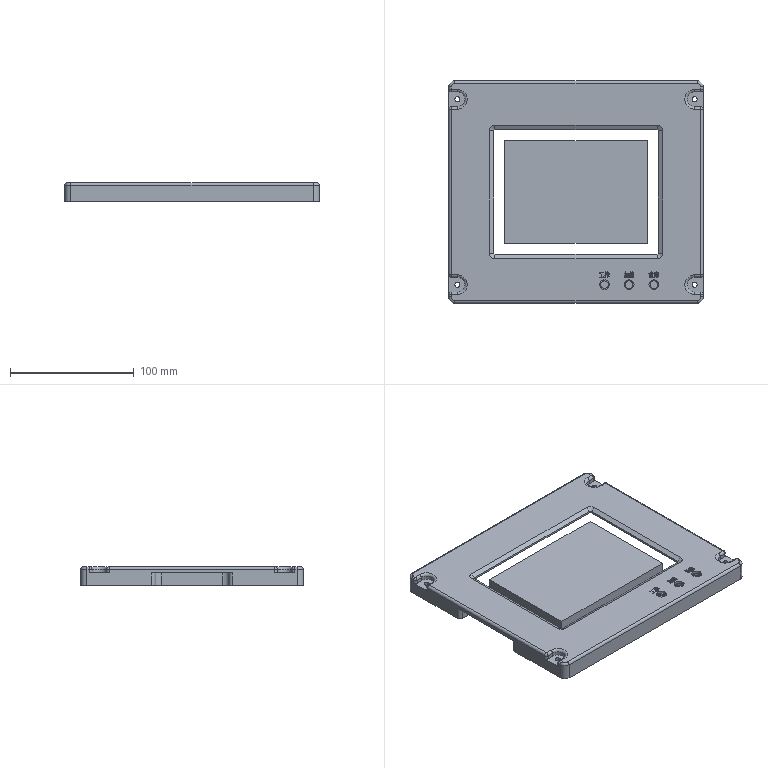NC program | Mastercam | posted with a generic post | part box 206 x 180 x 15 mm
Lines 14414 to 15524 of 42274:
(2 BM/BNOS |TOOL - 14|DIA. OFF. - 14|LEN. - 14|TOOL DIA. - 2.)
N9094 T14 M6
N9096 G0 G54 G90 X69.714 Y49.5 C0. B0. S10000 M3
N9098 G43 H14 Z24.866
N9100 Z4.866
N9102 G1 Z-.134 F600.
N9104 X69.698 Y49.856 F2000.
N9106 X69.648 Y50.221
N9108 X69.561 Y50.591
N9110 X69.436 Y50.959
N9112 X69.271 Y51.321
N9114 X69.068 Y51.669
N9116 X68.828 Y51.999
N9118 X68.553 Y52.303
N9120 X68.249 Y52.578
N9122 X67.919 Y52.818
N9124 X67.571 Y53.021
N9126 X67.209 Y53.186
N9128 X66.841 Y53.311
N9130 X66.471 Y53.398
N9132 X66.106 Y53.448
N9134 X65.75 Y53.464
N9136 X-65.75
N9138 X-66.106 Y53.448
N9140 X-66.471 Y53.398
N9142 X-66.841 Y53.311
N9144 X-67.209 Y53.186
N9146 X-67.571 Y53.021
N9148 X-67.919 Y52.818
N9150 X-68.249 Y52.578
N9152 X-68.553 Y52.303
N9154 X-68.828 Y51.999
N9156 X-69.068 Y51.669
N9158 X-69.271 Y51.321
N9160 X-69.436 Y50.959
N9162 X-69.561 Y50.591
N9164 X-69.648 Y50.221
N9166 X-69.698 Y49.856
N9168 X-69.714 Y49.5
N9170 Y-49.5
N9172 X-69.627
N9174 Z-.184
N9176 Y49.5
N9178 X-69.612 Y49.848
N9180 X-69.563 Y50.206
N9182 X-69.478 Y50.567
N9184 X-69.355 Y50.927
N9186 X-69.194 Y51.281
N9188 X-68.995 Y51.622
N9190 X-68.76 Y51.944
N9192 X-68.492 Y52.242
N9194 X-68.194 Y52.51
N9196 X-67.872 Y52.745
N9198 X-67.531 Y52.944
N9200 X-67.177 Y53.105
N9202 X-66.817 Y53.228
N9204 X-66.456 Y53.313
N9206 X-66.098 Y53.362
N9208 X-65.75 Y53.377
N9210 X65.75
N9212 X66.098 Y53.362
N9214 X66.456 Y53.313
N9216 X66.817 Y53.228
N9218 X67.177 Y53.105
N9220 X67.531 Y52.944
N9222 X67.872 Y52.745
N9224 X68.194 Y52.51
N9226 X68.492 Y52.242
N9228 X68.76 Y51.944
N9230 X68.995 Y51.622
N9232 X69.194 Y51.281
N9234 X69.355 Y50.927
N9236 X69.478 Y50.567
N9238 X69.563 Y50.206
N9240 X69.612 Y49.848
N9242 X69.627 Y49.5
N9244 Y-49.5
N9246 X69.612 Y-49.848
N9248 X69.563 Y-50.206
N9250 X69.478 Y-50.567
N9252 X69.355 Y-50.927
N9254 X69.194 Y-51.281
N9256 X68.995 Y-51.622
N9258 X68.76 Y-51.944
N9260 X68.492 Y-52.242
N9262 X68.194 Y-52.51
N9264 X67.872 Y-52.745
N9266 X67.531 Y-52.944
N9268 X67.177 Y-53.105
N9270 X66.817 Y-53.228
N9272 X66.456 Y-53.313
N9274 X66.098 Y-53.362
N9276 X65.75 Y-53.377
N9278 X-65.75
N9280 X-66.098 Y-53.362
N9282 X-66.456 Y-53.313
N9284 X-66.817 Y-53.228
N9286 X-67.177 Y-53.105
N9288 X-67.531 Y-52.944
N9290 X-67.872 Y-52.745
N9292 X-68.194 Y-52.51
N9294 X-68.492 Y-52.242
N9296 X-68.76 Y-51.944
N9298 X-68.995 Y-51.622
N9300 X-69.194 Y-51.281
N9302 X-69.355 Y-50.927
N9304 X-69.478 Y-50.567
N9306 X-69.563 Y-50.206
N9308 X-69.612 Y-49.848
N9310 X-69.627 Y-49.5
N9312 X-69.541
N9314 Z-.234
N9316 X-69.526 Y-49.841
N9318 X-69.478 Y-50.19
N9320 X-69.395 Y-50.543
N9322 X-69.275 Y-50.895
N9324 X-69.117 Y-51.241
N9326 X-68.923 Y-51.574
N9328 X-68.693 Y-51.889
N9330 X-68.431 Y-52.181
N9332 X-68.139 Y-52.443
N9334 X-67.824 Y-52.673
N9336 X-67.491 Y-52.867
N9338 X-67.145 Y-53.025
N9340 X-66.793 Y-53.145
N9342 X-66.44 Y-53.228
N9344 X-66.091 Y-53.276
N9346 X-65.75 Y-53.291
N9348 X65.75
N9350 X66.091 Y-53.276
N9352 X66.44 Y-53.228
N9354 X66.793 Y-53.145
N9356 X67.145 Y-53.025
N9358 X67.491 Y-52.867
N9360 X67.824 Y-52.673
N9362 X68.139 Y-52.443
N9364 X68.431 Y-52.181
N9366 X68.693 Y-51.889
N9368 X68.923 Y-51.574
N9370 X69.117 Y-51.241
N9372 X69.275 Y-50.895
N9374 X69.395 Y-50.543
N9376 X69.478 Y-50.19
N9378 X69.526 Y-49.841
N9380 X69.541 Y-49.5
N9382 Y49.5
N9384 X69.526 Y49.841
N9386 X69.478 Y50.19
N9388 X69.395 Y50.543
N9390 X69.275 Y50.895
N9392 X69.117 Y51.241
N9394 X68.923 Y51.574
N9396 X68.693 Y51.889
N9398 X68.431 Y52.181
N9400 X68.139 Y52.443
N9402 X67.824 Y52.673
N9404 X67.491 Y52.867
N9406 X67.145 Y53.025
N9408 X66.793 Y53.145
N9410 X66.44 Y53.228
N9412 X66.091 Y53.276
N9414 X65.75 Y53.291
N9416 X-65.75
N9418 X-66.091 Y53.276
N9420 X-66.44 Y53.228
N9422 X-66.793 Y53.145
N9424 X-67.145 Y53.025
N9426 X-67.491 Y52.867
N9428 X-67.824 Y52.673
N9430 X-68.139 Y52.443
N9432 X-68.431 Y52.181
N9434 X-68.693 Y51.889
N9436 X-68.923 Y51.574
N9438 X-69.117 Y51.241
N9440 X-69.275 Y50.895
N9442 X-69.395 Y50.543
N9444 X-69.478 Y50.19
N9446 X-69.526 Y49.841
N9448 X-69.541 Y49.5
N9450 Y-49.5
N9452 X-69.454
N9454 Z-.284
N9456 Y49.5
N9458 X-69.439 Y49.833
N9460 X-69.392 Y50.174
N9462 X-69.311 Y50.519
N9464 X-69.194 Y50.864
N9466 X-69.04 Y51.201
N9468 X-68.85 Y51.527
N9470 X-68.626 Y51.835
N9472 X-68.369 Y52.119
N9474 X-68.085 Y52.376
N9476 X-67.777 Y52.6
N9478 X-67.451 Y52.79
N9480 X-67.114 Y52.944
N9482 X-66.769 Y53.061
N9484 X-66.424 Y53.142
N9486 X-66.083 Y53.189
N9488 X-65.75 Y53.204
N9490 X65.75
N9492 X66.083 Y53.189
N9494 X66.424 Y53.142
N9496 X66.769 Y53.061
N9498 X67.114 Y52.944
N9500 X67.451 Y52.79
N9502 X67.777 Y52.6
N9504 X68.085 Y52.376
N9506 X68.369 Y52.119
N9508 X68.626 Y51.835
N9510 X68.85 Y51.527
N9512 X69.04 Y51.201
N9514 X69.194 Y50.864
N9516 X69.311 Y50.519
N9518 X69.392 Y50.174
N9520 X69.439 Y49.833
N9522 X69.454 Y49.5
N9524 Y-49.5
N9526 X69.439 Y-49.833
N9528 X69.392 Y-50.174
N9530 X69.311 Y-50.519
N9532 X69.194 Y-50.864
N9534 X69.04 Y-51.201
N9536 X68.85 Y-51.527
N9538 X68.626 Y-51.835
N9540 X68.369 Y-52.119
N9542 X68.085 Y-52.376
N9544 X67.777 Y-52.6
N9546 X67.451 Y-52.79
N9548 X67.114 Y-52.944
N9550 X66.769 Y-53.061
N9552 X66.424 Y-53.142
N9554 X66.083 Y-53.189
N9556 X65.75 Y-53.204
N9558 X-65.75
N9560 X-66.083 Y-53.189
N9562 X-66.424 Y-53.142
N9564 X-66.769 Y-53.061
N9566 X-67.114 Y-52.944
N9568 X-67.451 Y-52.79
N9570 X-67.777 Y-52.6
N9572 X-68.085 Y-52.376
N9574 X-68.369 Y-52.119
N9576 X-68.626 Y-51.835
N9578 X-68.85 Y-51.527
N9580 X-69.04 Y-51.201
N9582 X-69.194 Y-50.864
N9584 X-69.311 Y-50.519
N9586 X-69.392 Y-50.174
N9588 X-69.439 Y-49.833
N9590 X-69.454 Y-49.5
N9592 X-69.368
N9594 Z-.334
N9596 X-69.353 Y-49.825
N9598 X-69.307 Y-50.158
N9600 X-69.228 Y-50.495
N9602 X-69.114 Y-50.832
N9604 X-68.964 Y-51.162
N9606 X-68.778 Y-51.48
N9608 X-68.559 Y-51.78
N9610 X-68.308 Y-52.058
N9612 X-68.03 Y-52.309
N9614 X-67.73 Y-52.528
N9616 X-67.412 Y-52.714
N9618 X-67.082 Y-52.864
N9620 X-66.745 Y-52.978
N9622 X-66.408 Y-53.057
N9624 X-66.075 Y-53.103
N9626 X-65.75 Y-53.118
N9628 X65.75
N9630 X66.075 Y-53.103
N9632 X66.408 Y-53.057
N9634 X66.745 Y-52.978
N9636 X67.082 Y-52.864
N9638 X67.412 Y-52.714
N9640 X67.73 Y-52.528
N9642 X68.03 Y-52.309
N9644 X68.308 Y-52.058
N9646 X68.559 Y-51.78
N9648 X68.778 Y-51.48
N9650 X68.964 Y-51.162
N9652 X69.114 Y-50.832
N9654 X69.228 Y-50.495
N9656 X69.307 Y-50.158
N9658 X69.353 Y-49.825
N9660 X69.368 Y-49.5
N9662 Y49.5
N9664 X69.353 Y49.825
N9666 X69.307 Y50.158
N9668 X69.228 Y50.495
N9670 X69.114 Y50.832
N9672 X68.964 Y51.162
N9674 X68.778 Y51.48
N9676 X68.559 Y51.78
N9678 X68.308 Y52.058
N9680 X68.03 Y52.309
N9682 X67.73 Y52.528
N9684 X67.412 Y52.714
N9686 X67.082 Y52.864
N9688 X66.745 Y52.978
N9690 X66.408 Y53.057
N9692 X66.075 Y53.103
N9694 X65.75 Y53.118
N9696 X-65.75
N9698 X-66.075 Y53.103
N9700 X-66.408 Y53.057
N9702 X-66.745 Y52.978
N9704 X-67.082 Y52.864
N9706 X-67.412 Y52.714
N9708 X-67.73 Y52.528
N9710 X-68.03 Y52.309
N9712 X-68.308 Y52.058
N9714 X-68.559 Y51.78
N9716 X-68.778 Y51.48
N9718 X-68.964 Y51.162
N9720 X-69.114 Y50.832
N9722 X-69.228 Y50.495
N9724 X-69.307 Y50.158
N9726 X-69.353 Y49.825
N9728 X-69.368 Y49.5
N9730 Y-49.5
N9732 X-69.281
N9734 Z-.384
N9736 Y49.5
N9738 X-69.267 Y49.817
N9740 X-69.222 Y50.143
N9742 X-69.145 Y50.472
N9744 X-69.033 Y50.8
N9746 X-68.887 Y51.122
N9748 X-68.706 Y51.432
N9750 X-68.491 Y51.726
N9752 X-68.247 Y51.997
N9754 X-67.976 Y52.241
N9756 X-67.682 Y52.456
N9758 X-67.372 Y52.637
N9760 X-67.05 Y52.783
N9762 X-66.722 Y52.895
N9764 X-66.393 Y52.972
N9766 X-66.067 Y53.017
N9768 X-65.75 Y53.031
N9770 X65.75
N9772 X66.067 Y53.017
N9774 X66.393 Y52.972
N9776 X66.722 Y52.895
N9778 X67.05 Y52.783
N9780 X67.372 Y52.637
N9782 X67.682 Y52.456
N9784 X67.976 Y52.241
N9786 X68.247 Y51.997
N9788 X68.491 Y51.726
N9790 X68.706 Y51.432
N9792 X68.887 Y51.122
N9794 X69.033 Y50.8
N9796 X69.145 Y50.472
N9798 X69.222 Y50.143
N9800 X69.267 Y49.817
N9802 X69.281 Y49.5
N9804 Y-49.5
N9806 X69.267 Y-49.817
N9808 X69.222 Y-50.143
N9810 X69.145 Y-50.472
N9812 X69.033 Y-50.8
N9814 X68.887 Y-51.122
N9816 X68.706 Y-51.432
N9818 X68.491 Y-51.726
N9820 X68.247 Y-51.997
N9822 X67.976 Y-52.241
N9824 X67.682 Y-52.456
N9826 X67.372 Y-52.637
N9828 X67.05 Y-52.783
N9830 X66.722 Y-52.895
N9832 X66.393 Y-52.972
N9834 X66.067 Y-53.017
N9836 X65.75 Y-53.031
N9838 X-65.75
N9840 X-66.067 Y-53.017
N9842 X-66.393 Y-52.972
N9844 X-66.722 Y-52.895
N9846 X-67.05 Y-52.783
N9848 X-67.372 Y-52.637
N9850 X-67.682 Y-52.456
N9852 X-67.976 Y-52.241
N9854 X-68.247 Y-51.997
N9856 X-68.491 Y-51.726
N9858 X-68.706 Y-51.432
N9860 X-68.887 Y-51.122
N9862 X-69.033 Y-50.8
N9864 X-69.145 Y-50.472
N9866 X-69.222 Y-50.143
N9868 X-69.267 Y-49.817
N9870 X-69.281 Y-49.5
N9872 X-69.194
N9874 Z-.434
N9876 X-69.181 Y-49.81
N9878 X-69.137 Y-50.127
N9880 X-69.062 Y-50.448
N9882 X-68.953 Y-50.768
N9884 X-68.81 Y-51.082
N9886 X-68.633 Y-51.385
N9888 X-68.424 Y-51.671
N9890 X-68.186 Y-51.936
N9892 X-67.921 Y-52.174
N9894 X-67.635 Y-52.383
N9896 X-67.332 Y-52.56
N9898 X-67.018 Y-52.703
N9900 X-66.698 Y-52.812
N9902 X-66.377 Y-52.887
N9904 X-66.06 Y-52.931
N9906 X-65.75 Y-52.944
N9908 X65.75
N9910 X66.06 Y-52.931
N9912 X66.377 Y-52.887
N9914 X66.698 Y-52.812
N9916 X67.018 Y-52.703
N9918 X67.332 Y-52.56
N9920 X67.635 Y-52.383
N9922 X67.921 Y-52.174
N9924 X68.186 Y-51.936
N9926 X68.424 Y-51.671
N9928 X68.633 Y-51.385
N9930 X68.81 Y-51.082
N9932 X68.953 Y-50.768
N9934 X69.062 Y-50.448
N9936 X69.137 Y-50.127
N9938 X69.181 Y-49.81
N9940 X69.194 Y-49.5
N9942 Y49.5
N9944 X69.181 Y49.81
N9946 X69.137 Y50.127
N9948 X69.062 Y50.448
N9950 X68.953 Y50.768
N9952 X68.81 Y51.082
N9954 X68.633 Y51.385
N9956 X68.424 Y51.671
N9958 X68.186 Y51.936
N9960 X67.921 Y52.174
N9962 X67.635 Y52.383
N9964 X67.332 Y52.56
N9966 X67.018 Y52.703
N9968 X66.698 Y52.812
N9970 X66.377 Y52.887
N9972 X66.06 Y52.931
N9974 X65.75 Y52.944
N9976 X-65.75
N9978 X-66.06 Y52.931
N9980 X-66.377 Y52.887
N9982 X-66.698 Y52.812
N9984 X-67.018 Y52.703
N9986 X-67.332 Y52.56
N9988 X-67.635 Y52.383
N9990 X-67.921 Y52.174
N9992 X-68.186 Y51.936
N9994 X-68.424 Y51.671
N9996 X-68.633 Y51.385
N9998 X-68.81 Y51.082
N100 X-68.953 Y50.768
N102 X-69.062 Y50.448
N104 X-69.137 Y50.127
N106 X-69.181 Y49.81
N108 X-69.194 Y49.5
N110 Y-49.5
N112 X-69.108
N114 Z-.484
N116 Y49.5
N118 X-69.094 Y49.802
N120 X-69.052 Y50.111
N122 X-68.978 Y50.424
N124 X-68.872 Y50.736
N126 X-68.733 Y51.042
N128 X-68.561 Y51.337
N130 X-68.357 Y51.616
N132 X-68.124 Y51.874
N134 X-67.866 Y52.107
N136 X-67.587 Y52.311
N138 X-67.292 Y52.483
N140 X-66.986 Y52.622
N142 X-66.674 Y52.728
N144 X-66.361 Y52.802
N146 X-66.052 Y52.844
N148 X-65.75 Y52.858
N150 X65.75
N152 X66.052 Y52.844
N154 X66.361 Y52.802
N156 X66.674 Y52.728
N158 X66.986 Y52.622
N160 X67.292 Y52.483
N162 X67.587 Y52.311
N164 X67.866 Y52.107
N166 X68.124 Y51.874
N168 X68.357 Y51.616
N170 X68.561 Y51.337
N172 X68.733 Y51.042
N174 X68.872 Y50.736
N176 X68.978 Y50.424
N178 X69.052 Y50.111
N180 X69.094 Y49.802
N182 X69.108 Y49.5
N184 Y-49.5
N186 X69.094 Y-49.802
N188 X69.052 Y-50.111
N190 X68.978 Y-50.424
N192 X68.872 Y-50.736
N194 X68.733 Y-51.042
N196 X68.561 Y-51.337
N198 X68.357 Y-51.616
N200 X68.124 Y-51.874
N202 X67.866 Y-52.107
N204 X67.587 Y-52.311
N206 X67.292 Y-52.483
N208 X66.986 Y-52.622
N210 X66.674 Y-52.728
N212 X66.361 Y-52.802
N214 X66.052 Y-52.844
N216 X65.75 Y-52.858
N218 X-65.75
N220 X-66.052 Y-52.844
N222 X-66.361 Y-52.802
N224 X-66.674 Y-52.728
N226 X-66.986 Y-52.622
N228 X-67.292 Y-52.483
N230 X-67.587 Y-52.311
N232 X-67.866 Y-52.107
N234 X-68.124 Y-51.874
N236 X-68.357 Y-51.616
N238 X-68.561 Y-51.337
N240 X-68.733 Y-51.042
N242 X-68.872 Y-50.736
N244 X-68.978 Y-50.424
N246 X-69.052 Y-50.111
N248 X-69.094 Y-49.802
N250 X-69.108 Y-49.5
N252 X-69.021
N254 Z-.534
N256 X-69.008 Y-49.794
N258 X-68.967 Y-50.095
N260 X-68.895 Y-50.4
N262 X-68.792 Y-50.704
N264 X-68.656 Y-51.002
N266 X-68.488 Y-51.29
N268 X-68.29 Y-51.562
N270 X-68.063 Y-51.813
N272 X-67.812 Y-52.04
N274 X-67.54 Y-52.238
N276 X-67.252 Y-52.406
N278 X-66.954 Y-52.542
N280 X-66.65 Y-52.645
N282 X-66.345 Y-52.717
N284 X-66.044 Y-52.758
N286 X-65.75 Y-52.771
N288 X65.75
N290 X66.044 Y-52.758
N292 X66.345 Y-52.717
N294 X66.65 Y-52.645
N296 X66.954 Y-52.542
N298 X67.252 Y-52.406
N300 X67.54 Y-52.238
N302 X67.812 Y-52.04
N304 X68.063 Y-51.813
N306 X68.29 Y-51.562
N308 X68.488 Y-51.29
N310 X68.656 Y-51.002
N312 X68.792 Y-50.704
N314 X68.895 Y-50.4
N316 X68.967 Y-50.095
N318 X69.008 Y-49.794
N320 X69.021 Y-49.5
N322 Y49.5
N324 X69.008 Y49.794
N326 X68.967 Y50.095
N328 X68.895 Y50.4
N330 X68.792 Y50.704
N332 X68.656 Y51.002
N334 X68.488 Y51.29
N336 X68.29 Y51.562
N338 X68.063 Y51.813
N340 X67.812 Y52.04
N342 X67.54 Y52.238
N344 X67.252 Y52.406
N346 X66.954 Y52.542
N348 X66.65 Y52.645
N350 X66.345 Y52.717
N352 X66.044 Y52.758
N354 X65.75 Y52.771
N356 X-65.75
N358 X-66.044 Y52.758
N360 X-66.345 Y52.717
N362 X-66.65 Y52.645
N364 X-66.954 Y52.542
N366 X-67.252 Y52.406
N368 X-67.54 Y52.238
N370 X-67.812 Y52.04
N372 X-68.063 Y51.813
N374 X-68.29 Y51.562
N376 X-68.488 Y51.29
N378 X-68.656 Y51.002
N380 X-68.792 Y50.704
N382 X-68.895 Y50.4
N384 X-68.967 Y50.095
N386 X-69.008 Y49.794
N388 X-69.021 Y49.5
N390 Y-49.5
N392 X-68.935
N394 Z-.584
N396 Y49.5
N398 X-68.922 Y49.786
N400 X-68.882 Y50.079
N402 X-68.812 Y50.376
N404 X-68.711 Y50.672
N406 X-68.579 Y50.963
N408 X-68.416 Y51.243
N410 X-68.222 Y51.507
N412 X-68.002 Y51.752
N414 X-67.757 Y51.972
N416 X-67.493 Y52.166
N418 X-67.213 Y52.329
N420 X-66.922 Y52.461
N422 X-66.626 Y52.562
N424 X-66.329 Y52.632
N426 X-66.036 Y52.672
N428 X-65.75 Y52.685
N430 X65.75
N432 X66.036 Y52.672
N434 X66.329 Y52.632
N436 X66.626 Y52.562
N438 X66.922 Y52.461
N440 X67.213 Y52.329
N442 X67.493 Y52.166
N444 X67.757 Y51.972
N446 X68.002 Y51.752
N448 X68.222 Y51.507
N450 X68.416 Y51.243
N452 X68.579 Y50.963
N454 X68.711 Y50.672
N456 X68.812 Y50.376
N458 X68.882 Y50.079
N460 X68.922 Y49.786
N462 X68.935 Y49.5
N464 Y-49.5
N466 X68.922 Y-49.786
N468 X68.882 Y-50.079
N470 X68.812 Y-50.376
N472 X68.711 Y-50.672
N474 X68.579 Y-50.963
N476 X68.416 Y-51.243
N478 X68.222 Y-51.507
N480 X68.002 Y-51.752
N482 X67.757 Y-51.972
N484 X67.493 Y-52.166
N486 X67.213 Y-52.329
N488 X66.922 Y-52.461
N490 X66.626 Y-52.562
N492 X66.329 Y-52.632
N494 X66.036 Y-52.672
N496 X65.75 Y-52.685
N498 X-65.75
N500 X-66.036 Y-52.672
N502 X-66.329 Y-52.632
N504 X-66.626 Y-52.562
N506 X-66.922 Y-52.461
N508 X-67.213 Y-52.329
N510 X-67.493 Y-52.166
N512 X-67.757 Y-51.972
N514 X-68.002 Y-51.752
N516 X-68.222 Y-51.507
N518 X-68.416 Y-51.243
N520 X-68.579 Y-50.963
N522 X-68.711 Y-50.672
N524 X-68.812 Y-50.376
N526 X-68.882 Y-50.079
N528 X-68.922 Y-49.786
N530 X-68.935 Y-49.5
N532 X-68.848
N534 Z-.634
N536 X-68.836 Y-49.778
N538 X-68.796 Y-50.064
N540 X-68.728 Y-50.352
N542 X-68.631 Y-50.64
N544 X-68.502 Y-50.923
N546 X-68.343 Y-51.195
N548 X-68.155 Y-51.453
N550 X-67.941 Y-51.691
N552 X-67.703 Y-51.905
N554 X-67.445 Y-52.093
N556 X-67.173 Y-52.252
N558 X-66.89 Y-52.381
N560 X-66.602 Y-52.478
N562 X-66.314 Y-52.546
N564 X-66.028 Y-52.586
N566 X-65.75 Y-52.598
N568 X65.75
N570 X66.028 Y-52.586
N572 X66.314 Y-52.546
N574 X66.602 Y-52.478
N576 X66.89 Y-52.381
N578 X67.173 Y-52.252
N580 X67.445 Y-52.093
N582 X67.703 Y-51.905
N584 X67.941 Y-51.691
N586 X68.155 Y-51.453
N588 X68.343 Y-51.195
N590 X68.502 Y-50.923
N592 X68.631 Y-50.64
N594 X68.728 Y-50.352
N596 X68.796 Y-50.064
N598 X68.836 Y-49.778
N600 X68.848 Y-49.5
N602 Y49.5
N604 X68.836 Y49.778
N606 X68.796 Y50.064
N608 X68.728 Y50.352
N610 X68.631 Y50.64
N612 X68.502 Y50.923
N614 X68.343 Y51.195
N616 X68.155 Y51.453
N618 X67.941 Y51.691
N620 X67.703 Y51.905
N622 X67.445 Y52.093
N624 X67.173 Y52.252
N626 X66.89 Y52.381
N628 X66.602 Y52.478
N630 X66.314 Y52.546
N632 X66.028 Y52.586
N634 X65.75 Y52.598
N636 X-65.75
N638 X-66.028 Y52.586
N640 X-66.314 Y52.546
N642 X-66.602 Y52.478
N644 X-66.89 Y52.381
N646 X-67.173 Y52.252
N648 X-67.445 Y52.093
N650 X-67.703 Y51.905
N652 X-67.941 Y51.691
N654 X-68.155 Y51.453
N656 X-68.343 Y51.195
N658 X-68.502 Y50.923
N660 X-68.631 Y50.64
N662 X-68.728 Y50.352
N664 X-68.796 Y50.064
N666 X-68.836 Y49.778
N668 X-68.848 Y49.5
N670 Y-49.5
N672 X-68.761
N674 Z-.684
N676 Y49.5
N678 X-68.749 Y49.771
N680 X-68.711 Y50.048
N682 X-68.645 Y50.329
N684 X-68.55 Y50.609
N686 X-68.425 Y50.883
N688 X-68.271 Y51.148
N690 X-68.088 Y51.398
N692 X-67.879 Y51.629
N694 X-67.648 Y51.838
N696 X-67.398 Y52.021
N698 X-67.133 Y52.175
N700 X-66.859 Y52.3
N702 X-66.579 Y52.395
N704 X-66.298 Y52.461
N706 X-66.021 Y52.499
N708 X-65.75 Y52.511
N710 X65.75
N712 X66.021 Y52.499
N714 X66.298 Y52.461
N716 X66.579 Y52.395
N718 X66.859 Y52.3
N720 X67.133 Y52.175
N722 X67.398 Y52.021
N724 X67.648 Y51.838
N726 X67.879 Y51.629
N728 X68.088 Y51.398
N730 X68.271 Y51.148
N732 X68.425 Y50.883
N734 X68.55 Y50.609
N736 X68.645 Y50.329
N738 X68.711 Y50.048
N740 X68.749 Y49.771
N742 X68.761 Y49.5
N744 Y-49.5
N746 X68.749 Y-49.771
N748 X68.711 Y-50.048
N750 X68.645 Y-50.329
N752 X68.55 Y-50.609
N754 X68.425 Y-50.883
N756 X68.271 Y-51.148
N758 X68.088 Y-51.398
N760 X67.879 Y-51.629
N762 X67.648 Y-51.838
N764 X67.398 Y-52.021
N766 X67.133 Y-52.175
N768 X66.859 Y-52.3
N770 X66.579 Y-52.395
N772 X66.298 Y-52.461
N774 X66.021 Y-52.499
N776 X65.75 Y-52.511
N778 X-65.75
N780 X-66.021 Y-52.499
N782 X-66.298 Y-52.461
N784 X-66.579 Y-52.395
N786 X-66.859 Y-52.3
N788 X-67.133 Y-52.175
N790 X-67.398 Y-52.021
N792 X-67.648 Y-51.838
N794 X-67.879 Y-51.629
N796 X-68.088 Y-51.398
N798 X-68.271 Y-51.148
N800 X-68.425 Y-50.883
N802 X-68.55 Y-50.609
N804 X-68.645 Y-50.329
N806 X-68.711 Y-50.048
N808 X-68.749 Y-49.771
N810 X-68.761 Y-49.5
N812 X-68.675
N814 Z-.734
N816 X-68.663 Y-49.763
N818 X-68.626 Y-50.032
N820 X-68.562 Y-50.305
N822 X-68.47 Y-50.577
N824 X-68.348 Y-50.843
N826 X-68.198 Y-51.101
N828 X-68.021 Y-51.344
N830 X-67.818 Y-51.568
N832 X-67.594 Y-51.771
N834 X-67.351 Y-51.948
N836 X-67.093 Y-52.098
N838 X-66.827 Y-52.22
N840 X-66.555 Y-52.312
N842 X-66.282 Y-52.376
N844 X-66.013 Y-52.413
N846 X-65.75 Y-52.425
N848 X65.75
N850 X66.013 Y-52.413
N852 X66.282 Y-52.376
N854 X66.555 Y-52.312
N856 X66.827 Y-52.22
N858 X67.093 Y-52.098
N860 X67.351 Y-51.948
N862 X67.594 Y-51.771
N864 X67.818 Y-51.568
N866 X68.021 Y-51.344
N868 X68.198 Y-51.101
N870 X68.348 Y-50.843
N872 X68.47 Y-50.577
N874 X68.562 Y-50.305
N876 X68.626 Y-50.032
N878 X68.663 Y-49.763
N880 X68.675 Y-49.5
N882 Y49.5
N884 X68.663 Y49.763
N886 X68.626 Y50.032
N888 X68.562 Y50.305
N890 X68.47 Y50.577
N892 X68.348 Y50.843
N894 X68.198 Y51.101
N896 X68.021 Y51.344
N898 X67.818 Y51.568
N900 X67.594 Y51.771
N902 X67.351 Y51.948
N904 X67.093 Y52.098
N906 X66.827 Y52.22
N908 X66.555 Y52.312
N910 X66.282 Y52.376
N912 X66.013 Y52.413
N914 X65.75 Y52.425
N916 X-65.75
N918 X-66.013 Y52.413
N920 X-66.282 Y52.376
N922 X-66.555 Y52.312
N924 X-66.827 Y52.22
N926 X-67.093 Y52.098
N928 X-67.351 Y51.948
N930 X-67.594 Y51.771
N932 X-67.818 Y51.568
N934 X-68.021 Y51.344
N936 X-68.198 Y51.101
N938 X-68.348 Y50.843
N940 X-68.47 Y50.577
N942 X-68.562 Y50.305
N944 X-68.626 Y50.032
N946 X-68.663 Y49.763
N948 X-68.675 Y49.5
N950 Y-49.5
N952 X-68.588
N954 Z-.784
N956 Y49.5
N958 X-68.577 Y49.755
N960 X-68.541 Y50.016
N962 X-68.479 Y50.281
N964 X-68.389 Y50.545
N966 X-68.271 Y50.804
N968 X-68.126 Y51.053
N970 X-67.953 Y51.289
N972 X-67.757 Y51.507
N974 X-67.539 Y51.703
N976 X-67.303 Y51.876
N978 X-67.054 Y52.021
N980 X-66.795 Y52.139
N982 X-66.531 Y52.229
N984 X-66.266 Y52.291
N986 X-66.005 Y52.327
N988 X-65.75 Y52.338
N990 X65.75
N992 X66.005 Y52.327
N994 X66.266 Y52.291
N996 X66.531 Y52.229
N998 X66.795 Y52.139
N1000 X67.054 Y52.021
N1002 X67.303 Y51.876
N1004 X67.539 Y51.703
N1006 X67.757 Y51.507
N1008 X67.953 Y51.289
N1010 X68.126 Y51.053
N1012 X68.271 Y50.804
N1014 X68.389 Y50.545
N1016 X68.479 Y50.281
N1018 X68.541 Y50.016
N1020 X68.577 Y49.755
N1022 X68.588 Y49.5
N1024 Y-49.5
N1026 X68.577 Y-49.755
N1028 X68.541 Y-50.016
N1030 X68.479 Y-50.281
N1032 X68.389 Y-50.545
N1034 X68.271 Y-50.804
N1036 X68.126 Y-51.053
N1038 X67.953 Y-51.289
N1040 X67.757 Y-51.507
N1042 X67.539 Y-51.703
N1044 X67.303 Y-51.876
N1046 X67.054 Y-52.021
N1048 X66.795 Y-52.139
N1050 X66.531 Y-52.229
N1052 X66.266 Y-52.291
N1054 X66.005 Y-52.327
N1056 X65.75 Y-52.338
N1058 X-65.75
N1060 X-66.005 Y-52.327
N1062 X-66.266 Y-52.291
N1064 X-66.531 Y-52.229
N1066 X-66.795 Y-52.139
N1068 X-67.054 Y-52.021
N1070 X-67.303 Y-51.876
N1072 X-67.539 Y-51.703
N1074 X-67.757 Y-51.507
N1076 X-67.953 Y-51.289
N1078 X-68.126 Y-51.053
N1080 X-68.271 Y-50.804
N1082 X-68.389 Y-50.545
N1084 X-68.479 Y-50.281
N1086 X-68.541 Y-50.016
N1088 X-68.577 Y-49.755
N1090 X-68.588 Y-49.5
N1092 X-68.502
N1094 Z-.834
N1096 X-68.491 Y-49.747
N1098 X-68.456 Y-50.001
N1100 X-68.395 Y-50.257
N1102 X-68.308 Y-50.513
N1104 X-68.194 Y-50.764
N1106 X-68.053 Y-51.006
N1108 X-67.886 Y-51.234
N1110 X-67.696 Y-51.446
N1112 X-67.484 Y-51.636
N1114 X-67.256 Y-51.803
N1116 X-67.014 Y-51.944
N1118 X-66.763 Y-52.058
N1120 X-66.507 Y-52.145
N1122 X-66.251 Y-52.206
N1124 X-65.997 Y-52.241
N1126 X-65.75 Y-52.252
N1128 X65.75
N1130 X65.997 Y-52.241
N1132 X66.251 Y-52.206
N1134 X66.507 Y-52.145
N1136 X66.763 Y-52.058
N1138 X67.014 Y-51.944
N1140 X67.256 Y-51.803
N1142 X67.484 Y-51.636
N1144 X67.696 Y-51.446
N1146 X67.886 Y-51.234
N1148 X68.053 Y-51.006
N1150 X68.194 Y-50.764
N1152 X68.308 Y-50.513
N1154 X68.395 Y-50.257
N1156 X68.456 Y-50.001
N1158 X68.491 Y-49.747
N1160 X68.502 Y-49.5
N1162 Y49.5
N1164 X68.491 Y49.747
N1166 X68.456 Y50.001
N1168 X68.395 Y50.257
N1170 X68.308 Y50.513
N1172 X68.194 Y50.764
N1174 X68.053 Y51.006
N1176 X67.886 Y51.234
N1178 X67.696 Y51.446
N1180 X67.484 Y51.636
N1182 X67.256 Y51.803
N1184 X67.014 Y51.944
N1186 X66.763 Y52.058
N1188 X66.507 Y52.145
N1190 X66.251 Y52.206
N1192 X65.997 Y52.241
N1194 X65.75 Y52.252
N1196 X-65.75
N1198 X-65.997 Y52.241
N1200 X-66.251 Y52.206
N1202 X-66.507 Y52.145
N1204 X-66.763 Y52.058
N1206 X-67.014 Y51.944
N1208 X-67.256 Y51.803
N1210 X-67.484 Y51.636
N1212 X-67.696 Y51.446
N1214 X-67.886 Y51.234
N1216 X-68.053 Y51.006
N1218 X-68.194 Y50.764
N1220 X-68.308 Y50.513
N1222 X-68.395 Y50.257
N1224 X-68.456 Y50.001
N1226 X-68.491 Y49.747
N1228 X-68.502 Y49.5
N1230 Y-49.5
N1232 X-68.415
N1234 Z-.884
N1236 Y49.5
N1238 X-68.404 Y49.739
N1240 X-68.371 Y49.985
N1242 X-68.312 Y50.233
N1244 X-68.228 Y50.481
N1246 X-68.117 Y50.724
N1248 X-67.981 Y50.958
N1250 X-67.819 Y51.18
N1252 X-67.634 Y51.384
N1254 X-67.43 Y51.569
N1256 X-67.208 Y51.731
N1258 X-66.974 Y51.867
N1260 X-66.731 Y51.978
N1262 X-66.483 Y52.062
N1264 X-66.235 Y52.121
N1266 X-65.989 Y52.154
N1268 X-65.75 Y52.165
N1270 X65.75
N1272 X65.989 Y52.154
N1274 X66.235 Y52.121
N1276 X66.483 Y52.062
N1278 X66.731 Y51.978
N1280 X66.974 Y51.867
N1282 X67.208 Y51.731
N1284 X67.43 Y51.569
N1286 X67.634 Y51.384
N1288 X67.819 Y51.18
N1290 X67.981 Y50.958
N1292 X68.117 Y50.724
N1294 X68.228 Y50.481
N1296 X68.312 Y50.233
N1298 X68.371 Y49.985
N1300 X68.404 Y49.739
N1302 X68.415 Y49.5
N1304 Y-49.5
N1306 X68.404 Y-49.739
N1308 X68.371 Y-49.985
N1310 X68.312 Y-50.233
N1312 X68.228 Y-50.481
N1314 X68.117 Y-50.724
N1316 X67.981 Y-50.958
N1318 X67.819 Y-51.18
N1320 X67.634 Y-51.384
N1322 X67.43 Y-51.569
N1324 X67.208 Y-51.731
N1326 X66.974 Y-51.867
N1328 X66.731 Y-51.978
N1330 X66.483 Y-52.062
N1332 X66.235 Y-52.121
N1334 X65.989 Y-52.154
N1336 X65.75 Y-52.165
N1338 X-65.75
N1340 X-65.989 Y-52.154
N1342 X-66.235 Y-52.121
N1344 X-66.483 Y-52.062
N1346 X-66.731 Y-51.978
N1348 X-66.974 Y-51.867
N1350 X-67.208 Y-51.731
N1352 X-67.43 Y-51.569
N1354 X-67.634 Y-51.384
N1356 X-67.819 Y-51.18
N1358 X-67.981 Y-50.958
N1360 X-68.117 Y-50.724
N1362 X-68.228 Y-50.481
N1364 X-68.312 Y-50.233
N1366 X-68.371 Y-49.985
N1368 X-68.404 Y-49.739
N1370 X-68.415 Y-49.5
N1372 X-68.328
N1374 Z-.934
N1376 X-68.318 Y-49.732
N1378 X-68.285 Y-49.969
N1380 X-68.229 Y-50.209
N1382 X-68.147 Y-50.449
N1384 X-68.04 Y-50.684
N1386 X-67.908 Y-50.911
N1388 X-67.752 Y-51.125
N1390 X-67.573 Y-51.323
N1392 X-67.375 Y-51.502
N1394 X-67.161 Y-51.658
N1396 X-66.934 Y-51.79
N1398 X-66.699 Y-51.897
N1400 X-66.459 Y-51.979
N1402 X-66.219 Y-52.035
N1404 X-65.982 Y-52.068
N1406 X-65.75 Y-52.078
N1408 X65.75
N1410 X65.982 Y-52.068
N1412 X66.219 Y-52.035